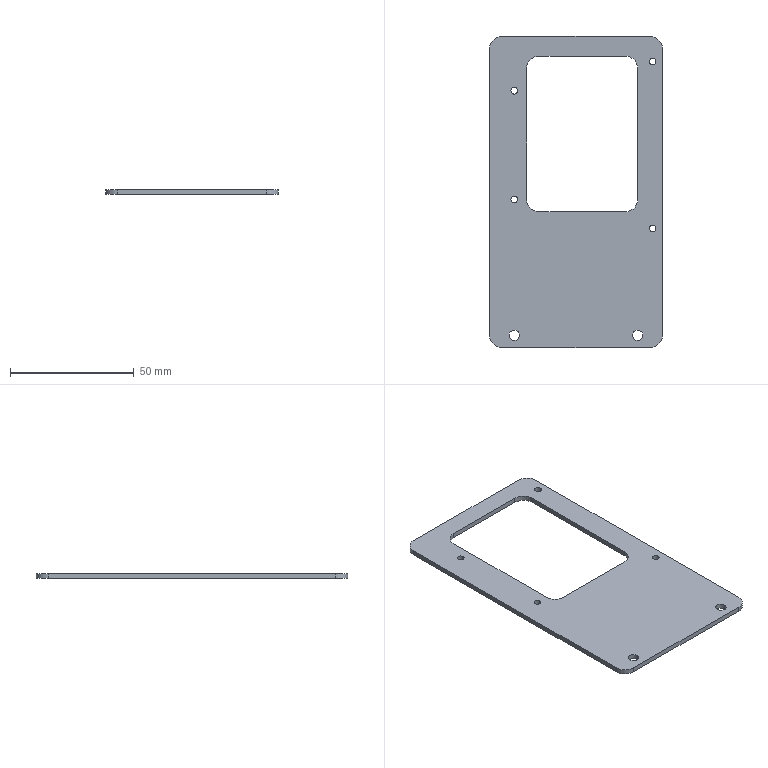Part | SolidWorks | features BaseBody 1 | 1 solid | 30 faces | box 70 x 126 x 2 mm | volume 11869 mm3 | cylinder 20 | plane 10 | commonest cylinder face diameters 2.7 x8 10 x8 4.2 x4
STEP:
#1=CARTESIAN_POINT('',(-27.1,-58.,0.));
#2=VERTEX_POINT('',#1);
#3=CARTESIAN_POINT('',(-22.9,-58.,0.));
#4=VERTEX_POINT('',#3);
#5=CARTESIAN_POINT('',(-25.,-58.,0.));
#6=DIRECTION('',(0.,0.,1.));
#7=DIRECTION('',(1.,0.,0.));
#8=AXIS2_PLACEMENT_3D('',#5,#6,#7);
#9=CIRCLE('',#8,2.1);
#10=EDGE_CURVE('',#2,#4,#9,.T.);
#11=ORIENTED_EDGE('',*,*,#10,.F.);
#12=CARTESIAN_POINT('',(-27.1,-58.,2.));
#13=VERTEX_POINT('',#12);
#14=CARTESIAN_POINT('',(-27.1,-58.,0.));
#15=DIRECTION('',(0.,0.,1.));
#16=VECTOR('',#15,1000.);
#17=LINE('',#14,#16);
#18=EDGE_CURVE('',#2,#13,#17,.T.);
#19=ORIENTED_EDGE('',*,*,#18,.T.);
#20=CARTESIAN_POINT('',(-22.9,-58.,2.));
#21=VERTEX_POINT('',#20);
#22=CARTESIAN_POINT('',(-25.,-58.,2.));
#23=DIRECTION('',(0.,0.,1.));
#24=DIRECTION('',(1.,0.,0.));
#25=AXIS2_PLACEMENT_3D('',#22,#23,#24);
#26=CIRCLE('',#25,2.1);
#27=EDGE_CURVE('',#13,#21,#26,.T.);
#28=ORIENTED_EDGE('',*,*,#27,.T.);
#29=CARTESIAN_POINT('',(-22.9,-58.,0.));
#30=DIRECTION('',(0.,0.,1.));
#31=VECTOR('',#30,1000.);
#32=LINE('',#29,#31);
#33=EDGE_CURVE('',#4,#21,#32,.T.);
#34=ORIENTED_EDGE('',*,*,#33,.F.);
#35=EDGE_LOOP('',(#11,#19,#28,#34));
#36=FACE_OUTER_BOUND('',#35,.T.);
#37=CARTESIAN_POINT('',(-25.,-58.,0.));
#38=DIRECTION('',(0.,0.,1.));
#39=DIRECTION('',(1.,0.,0.));
#40=AXIS2_PLACEMENT_3D('',#37,#38,#39);
#41=CYLINDRICAL_SURFACE('',#40,2.1);
#42=ADVANCED_FACE('',(#36),#41,.F.);
#43=CARTESIAN_POINT('',(29.65,-14.75,0.));
#44=VERTEX_POINT('',#43);
#45=CARTESIAN_POINT('',(32.35,-14.75,0.));
#46=VERTEX_POINT('',#45);
#47=CARTESIAN_POINT('',(31.,-14.75,0.));
#48=DIRECTION('',(0.,0.,1.));
#49=DIRECTION('',(1.,0.,0.));
#50=AXIS2_PLACEMENT_3D('',#47,#48,#49);
#51=CIRCLE('',#50,1.35);
#52=EDGE_CURVE('',#44,#46,#51,.T.);
#53=ORIENTED_EDGE('',*,*,#52,.F.);
#54=CARTESIAN_POINT('',(29.65,-14.75,2.));
#55=VERTEX_POINT('',#54);
#56=CARTESIAN_POINT('',(29.65,-14.75,0.));
#57=DIRECTION('',(0.,0.,1.));
#58=VECTOR('',#57,1000.);
#59=LINE('',#56,#58);
#60=EDGE_CURVE('',#44,#55,#59,.T.);
#61=ORIENTED_EDGE('',*,*,#60,.T.);
#62=CARTESIAN_POINT('',(32.35,-14.75,2.));
#63=VERTEX_POINT('',#62);
#64=CARTESIAN_POINT('',(31.,-14.75,2.));
#65=DIRECTION('',(0.,0.,1.));
#66=DIRECTION('',(1.,0.,0.));
#67=AXIS2_PLACEMENT_3D('',#64,#65,#66);
#68=CIRCLE('',#67,1.35);
#69=EDGE_CURVE('',#55,#63,#68,.T.);
#70=ORIENTED_EDGE('',*,*,#69,.T.);
#71=CARTESIAN_POINT('',(32.35,-14.75,0.));
#72=DIRECTION('',(0.,0.,1.));
#73=VECTOR('',#72,1000.);
#74=LINE('',#71,#73);
#75=EDGE_CURVE('',#46,#63,#74,.T.);
#76=ORIENTED_EDGE('',*,*,#75,.F.);
#77=EDGE_LOOP('',(#53,#61,#70,#76));
#78=FACE_OUTER_BOUND('',#77,.T.);
#79=CARTESIAN_POINT('',(31.,-14.75,0.));
#80=DIRECTION('',(0.,0.,1.));
#81=DIRECTION('',(1.,0.,0.));
#82=AXIS2_PLACEMENT_3D('',#79,#80,#81);
#83=CYLINDRICAL_SURFACE('',#82,1.35);
#84=ADVANCED_FACE('',(#78),#83,.F.);
#85=CARTESIAN_POINT('',(-26.35,41.,0.));
#86=VERTEX_POINT('',#85);
#87=CARTESIAN_POINT('',(-23.65,41.,0.));
#88=VERTEX_POINT('',#87);
#89=CARTESIAN_POINT('',(-25.,41.,0.));
#90=DIRECTION('',(0.,0.,1.));
#91=DIRECTION('',(1.,0.,0.));
#92=AXIS2_PLACEMENT_3D('',#89,#90,#91);
#93=CIRCLE('',#92,1.35);
#94=EDGE_CURVE('',#86,#88,#93,.T.);
#95=ORIENTED_EDGE('',*,*,#94,.F.);
#96=CARTESIAN_POINT('',(-26.35,41.,2.));
#97=VERTEX_POINT('',#96);
#98=CARTESIAN_POINT('',(-26.35,41.,0.));
#99=DIRECTION('',(0.,0.,1.));
#100=VECTOR('',#99,1000.);
#101=LINE('',#98,#100);
#102=EDGE_CURVE('',#86,#97,#101,.T.);
#103=ORIENTED_EDGE('',*,*,#102,.T.);
#104=CARTESIAN_POINT('',(-23.65,41.,2.));
#105=VERTEX_POINT('',#104);
#106=CARTESIAN_POINT('',(-25.,41.,2.));
#107=DIRECTION('',(0.,0.,1.));
#108=DIRECTION('',(1.,0.,0.));
#109=AXIS2_PLACEMENT_3D('',#106,#107,#108);
#110=CIRCLE('',#109,1.35);
#111=EDGE_CURVE('',#97,#105,#110,.T.);
#112=ORIENTED_EDGE('',*,*,#111,.T.);
#113=CARTESIAN_POINT('',(-23.65,41.,0.));
#114=DIRECTION('',(0.,0.,1.));
#115=VECTOR('',#114,1000.);
#116=LINE('',#113,#115);
#117=EDGE_CURVE('',#88,#105,#116,.T.);
#118=ORIENTED_EDGE('',*,*,#117,.F.);
#119=EDGE_LOOP('',(#95,#103,#112,#118));
#120=FACE_OUTER_BOUND('',#119,.T.);
#121=CARTESIAN_POINT('',(-25.,41.,0.));
#122=DIRECTION('',(0.,0.,1.));
#123=DIRECTION('',(1.,0.,0.));
#124=AXIS2_PLACEMENT_3D('',#121,#122,#123);
#125=CYLINDRICAL_SURFACE('',#124,1.35);
#126=ADVANCED_FACE('',(#120),#125,.F.);
#127=CARTESIAN_POINT('',(-26.35,-3.,0.));
#128=VERTEX_POINT('',#127);
#129=CARTESIAN_POINT('',(-23.65,-3.,0.));
#130=VERTEX_POINT('',#129);
#131=CARTESIAN_POINT('',(-25.,-3.,0.));
#132=DIRECTION('',(0.,0.,1.));
#133=DIRECTION('',(1.,0.,0.));
#134=AXIS2_PLACEMENT_3D('',#131,#132,#133);
#135=CIRCLE('',#134,1.35);
#136=EDGE_CURVE('',#128,#130,#135,.T.);
#137=ORIENTED_EDGE('',*,*,#136,.F.);
#138=CARTESIAN_POINT('',(-26.35,-3.,2.));
#139=VERTEX_POINT('',#138);
#140=CARTESIAN_POINT('',(-26.35,-3.,0.));
#141=DIRECTION('',(0.,0.,1.));
#142=VECTOR('',#141,1000.);
#143=LINE('',#140,#142);
#144=EDGE_CURVE('',#128,#139,#143,.T.);
#145=ORIENTED_EDGE('',*,*,#144,.T.);
#146=CARTESIAN_POINT('',(-23.65,-3.,2.));
#147=VERTEX_POINT('',#146);
#148=CARTESIAN_POINT('',(-25.,-3.,2.));
#149=DIRECTION('',(0.,0.,1.));
#150=DIRECTION('',(1.,0.,0.));
#151=AXIS2_PLACEMENT_3D('',#148,#149,#150);
#152=CIRCLE('',#151,1.35);
#153=EDGE_CURVE('',#139,#147,#152,.T.);
#154=ORIENTED_EDGE('',*,*,#153,.T.);
#155=CARTESIAN_POINT('',(-23.65,-3.,0.));
#156=DIRECTION('',(0.,0.,1.));
#157=VECTOR('',#156,1000.);
#158=LINE('',#155,#157);
#159=EDGE_CURVE('',#130,#147,#158,.T.);
#160=ORIENTED_EDGE('',*,*,#159,.F.);
#161=EDGE_LOOP('',(#137,#145,#154,#160));
#162=FACE_OUTER_BOUND('',#161,.T.);
#163=CARTESIAN_POINT('',(-25.,-3.,0.));
#164=DIRECTION('',(0.,0.,1.));
#165=DIRECTION('',(1.,0.,0.));
#166=AXIS2_PLACEMENT_3D('',#163,#164,#165);
#167=CYLINDRICAL_SURFACE('',#166,1.35);
#168=ADVANCED_FACE('',(#162),#167,.F.);
#169=CARTESIAN_POINT('',(22.9,-58.,0.));
#170=VERTEX_POINT('',#169);
#171=CARTESIAN_POINT('',(27.1,-58.,0.));
#172=VERTEX_POINT('',#171);
#173=CARTESIAN_POINT('',(25.,-58.,0.));
#174=DIRECTION('',(0.,0.,1.));
#175=DIRECTION('',(1.,0.,0.));
#176=AXIS2_PLACEMENT_3D('',#173,#174,#175);
#177=CIRCLE('',#176,2.1);
#178=EDGE_CURVE('',#170,#172,#177,.T.);
#179=ORIENTED_EDGE('',*,*,#178,.F.);
#180=CARTESIAN_POINT('',(22.9,-58.,2.));
#181=VERTEX_POINT('',#180);
#182=CARTESIAN_POINT('',(22.9,-58.,0.));
#183=DIRECTION('',(0.,0.,1.));
#184=VECTOR('',#183,1000.);
#185=LINE('',#182,#184);
#186=EDGE_CURVE('',#170,#181,#185,.T.);
#187=ORIENTED_EDGE('',*,*,#186,.T.);
#188=CARTESIAN_POINT('',(27.1,-58.,2.));
#189=VERTEX_POINT('',#188);
#190=CARTESIAN_POINT('',(25.,-58.,2.));
#191=DIRECTION('',(0.,0.,1.));
#192=DIRECTION('',(1.,0.,0.));
#193=AXIS2_PLACEMENT_3D('',#190,#191,#192);
#194=CIRCLE('',#193,2.1);
#195=EDGE_CURVE('',#181,#189,#194,.T.);
#196=ORIENTED_EDGE('',*,*,#195,.T.);
#197=CARTESIAN_POINT('',(27.1,-58.,0.));
#198=DIRECTION('',(0.,0.,1.));
#199=VECTOR('',#198,1000.);
#200=LINE('',#197,#199);
#201=EDGE_CURVE('',#172,#189,#200,.T.);
#202=ORIENTED_EDGE('',*,*,#201,.F.);
#203=EDGE_LOOP('',(#179,#187,#196,#202));
#204=FACE_OUTER_BOUND('',#203,.T.);
#205=CARTESIAN_POINT('',(25.,-58.,0.));
#206=DIRECTION('',(0.,0.,1.));
#207=DIRECTION('',(1.,0.,0.));
#208=AXIS2_PLACEMENT_3D('',#205,#206,#207);
#209=CYLINDRICAL_SURFACE('',#208,2.1);
#210=ADVANCED_FACE('',(#204),#209,.F.);
#211=CARTESIAN_POINT('',(29.65,52.75,0.));
#212=VERTEX_POINT('',#211);
#213=CARTESIAN_POINT('',(32.35,52.75,0.));
#214=VERTEX_POINT('',#213);
#215=CARTESIAN_POINT('',(31.,52.75,0.));
#216=DIRECTION('',(0.,0.,1.));
#217=DIRECTION('',(1.,0.,0.));
#218=AXIS2_PLACEMENT_3D('',#215,#216,#217);
#219=CIRCLE('',#218,1.35);
#220=EDGE_CURVE('',#212,#214,#219,.T.);
#221=ORIENTED_EDGE('',*,*,#220,.F.);
#222=CARTESIAN_POINT('',(29.65,52.75,2.));
#223=VERTEX_POINT('',#222);
#224=CARTESIAN_POINT('',(29.65,52.75,0.));
#225=DIRECTION('',(0.,0.,1.));
#226=VECTOR('',#225,1000.);
#227=LINE('',#224,#226);
#228=EDGE_CURVE('',#212,#223,#227,.T.);
#229=ORIENTED_EDGE('',*,*,#228,.T.);
#230=CARTESIAN_POINT('',(32.35,52.75,2.));
#231=VERTEX_POINT('',#230);
#232=CARTESIAN_POINT('',(31.,52.75,2.));
#233=DIRECTION('',(0.,0.,1.));
#234=DIRECTION('',(1.,0.,0.));
#235=AXIS2_PLACEMENT_3D('',#232,#233,#234);
#236=CIRCLE('',#235,1.35);
#237=EDGE_CURVE('',#223,#231,#236,.T.);
#238=ORIENTED_EDGE('',*,*,#237,.T.);
#239=CARTESIAN_POINT('',(32.35,52.75,0.));
#240=DIRECTION('',(0.,0.,1.));
#241=VECTOR('',#240,1000.);
#242=LINE('',#239,#241);
#243=EDGE_CURVE('',#214,#231,#242,.T.);
#244=ORIENTED_EDGE('',*,*,#243,.F.);
#245=EDGE_LOOP('',(#221,#229,#238,#244));
#246=FACE_OUTER_BOUND('',#245,.T.);
#247=CARTESIAN_POINT('',(31.,52.75,0.));
#248=DIRECTION('',(0.,0.,1.));
#249=DIRECTION('',(1.,0.,0.));
#250=AXIS2_PLACEMENT_3D('',#247,#248,#249);
#251=CYLINDRICAL_SURFACE('',#250,1.35);
#252=ADVANCED_FACE('',(#246),#251,.F.);
#253=CARTESIAN_POINT('',(35.,-58.,2.));
#254=VERTEX_POINT('',#253);
#255=CARTESIAN_POINT('',(30.,-63.,2.));
#256=VERTEX_POINT('',#255);
#257=CARTESIAN_POINT('',(30.,-58.,2.));
#258=DIRECTION('',(0.,0.,-1.));
#259=DIRECTION('',(-1.,0.,0.));
#260=AXIS2_PLACEMENT_3D('',#257,#258,#259);
#261=CIRCLE('',#260,5.);
#262=EDGE_CURVE('',#254,#256,#261,.T.);
#263=ORIENTED_EDGE('',*,*,#262,.F.);
#264=CARTESIAN_POINT('',(35.,58.,2.));
#265=VERTEX_POINT('',#264);
#266=CARTESIAN_POINT('',(35.,0.,2.));
#267=DIRECTION('',(0.,-1.,0.));
#268=VECTOR('',#267,1000.);
#269=LINE('',#266,#268);
#270=EDGE_CURVE('',#265,#254,#269,.T.);
#271=ORIENTED_EDGE('',*,*,#270,.F.);
#272=CARTESIAN_POINT('',(30.,63.,2.));
#273=VERTEX_POINT('',#272);
#274=CARTESIAN_POINT('',(30.,58.,2.));
#275=DIRECTION('',(0.,0.,-1.));
#276=DIRECTION('',(-1.,0.,0.));
#277=AXIS2_PLACEMENT_3D('',#274,#275,#276);
#278=CIRCLE('',#277,5.);
#279=EDGE_CURVE('',#273,#265,#278,.T.);
#280=ORIENTED_EDGE('',*,*,#279,.F.);
#281=CARTESIAN_POINT('',(-30.,63.,2.));
#282=VERTEX_POINT('',#281);
#283=CARTESIAN_POINT('',(0.,63.,2.));
#284=DIRECTION('',(1.,0.,0.));
#285=VECTOR('',#284,1000.);
#286=LINE('',#283,#285);
#287=EDGE_CURVE('',#282,#273,#286,.T.);
#288=ORIENTED_EDGE('',*,*,#287,.F.);
#289=CARTESIAN_POINT('',(-35.,58.,2.));
#290=VERTEX_POINT('',#289);
#291=CARTESIAN_POINT('',(-30.,58.,2.));
#292=DIRECTION('',(0.,0.,-1.));
#293=DIRECTION('',(-1.,0.,0.));
#294=AXIS2_PLACEMENT_3D('',#291,#292,#293);
#295=CIRCLE('',#294,5.);
#296=EDGE_CURVE('',#290,#282,#295,.T.);
#297=ORIENTED_EDGE('',*,*,#296,.F.);
#298=CARTESIAN_POINT('',(-35.,-58.,2.));
#299=VERTEX_POINT('',#298);
#300=CARTESIAN_POINT('',(-35.,0.,2.));
#301=DIRECTION('',(0.,1.,0.));
#302=VECTOR('',#301,1000.);
#303=LINE('',#300,#302);
#304=EDGE_CURVE('',#299,#290,#303,.T.);
#305=ORIENTED_EDGE('',*,*,#304,.F.);
#306=CARTESIAN_POINT('',(-30.,-63.,2.));
#307=VERTEX_POINT('',#306);
#308=CARTESIAN_POINT('',(-30.,-58.,2.));
#309=DIRECTION('',(0.,0.,-1.));
#310=DIRECTION('',(-1.,0.,0.));
#311=AXIS2_PLACEMENT_3D('',#308,#309,#310);
#312=CIRCLE('',#311,5.);
#313=EDGE_CURVE('',#307,#299,#312,.T.);
#314=ORIENTED_EDGE('',*,*,#313,.F.);
#315=CARTESIAN_POINT('',(0.,-63.,2.));
#316=DIRECTION('',(-1.,0.,0.));
#317=VECTOR('',#316,1000.);
#318=LINE('',#315,#317);
#319=EDGE_CURVE('',#256,#307,#318,.T.);
#320=ORIENTED_EDGE('',*,*,#319,.F.);
#321=EDGE_LOOP('',(#263,#271,#280,#288,#297,#305,#314,#320));
#322=FACE_OUTER_BOUND('',#321,.T.);
#323=CARTESIAN_POINT('',(-25.,-58.,2.));
#324=DIRECTION('',(0.,0.,1.));
#325=DIRECTION('',(1.,0.,0.));
#326=AXIS2_PLACEMENT_3D('',#323,#324,#325);
#327=CIRCLE('',#326,2.1);
#328=EDGE_CURVE('',#21,#13,#327,.T.);
#329=ORIENTED_EDGE('',*,*,#328,.F.);
#330=ORIENTED_EDGE('',*,*,#27,.F.);
#331=EDGE_LOOP('',(#329,#330));
#332=FACE_BOUND('',#331,.T.);
#333=CARTESIAN_POINT('',(31.,-14.75,2.));
#334=DIRECTION('',(0.,0.,1.));
#335=DIRECTION('',(1.,0.,0.));
#336=AXIS2_PLACEMENT_3D('',#333,#334,#335);
#337=CIRCLE('',#336,1.35);
#338=EDGE_CURVE('',#63,#55,#337,.T.);
#339=ORIENTED_EDGE('',*,*,#338,.F.);
#340=ORIENTED_EDGE('',*,*,#69,.F.);
#341=EDGE_LOOP('',(#339,#340));
#342=FACE_BOUND('',#341,.T.);
#343=CARTESIAN_POINT('',(-25.,41.,2.));
#344=DIRECTION('',(0.,0.,1.));
#345=DIRECTION('',(1.,0.,0.));
#346=AXIS2_PLACEMENT_3D('',#343,#344,#345);
#347=CIRCLE('',#346,1.35);
#348=EDGE_CURVE('',#105,#97,#347,.T.);
#349=ORIENTED_EDGE('',*,*,#348,.F.);
#350=ORIENTED_EDGE('',*,*,#111,.F.);
#351=EDGE_LOOP('',(#349,#350));
#352=FACE_BOUND('',#351,.T.);
#353=CARTESIAN_POINT('',(-25.,-3.,2.));
#354=DIRECTION('',(0.,0.,1.));
#355=DIRECTION('',(1.,0.,0.));
#356=AXIS2_PLACEMENT_3D('',#353,#354,#355);
#357=CIRCLE('',#356,1.35);
#358=EDGE_CURVE('',#147,#139,#357,.T.);
#359=ORIENTED_EDGE('',*,*,#358,.F.);
#360=ORIENTED_EDGE('',*,*,#153,.F.);
#361=EDGE_LOOP('',(#359,#360));
#362=FACE_BOUND('',#361,.T.);
#363=CARTESIAN_POINT('',(25.,-58.,2.));
#364=DIRECTION('',(0.,0.,1.));
#365=DIRECTION('',(1.,0.,0.));
#366=AXIS2_PLACEMENT_3D('',#363,#364,#365);
#367=CIRCLE('',#366,2.1);
#368=EDGE_CURVE('',#189,#181,#367,.T.);
#369=ORIENTED_EDGE('',*,*,#368,.F.);
#370=ORIENTED_EDGE('',*,*,#195,.F.);
#371=EDGE_LOOP('',(#369,#370));
#372=FACE_BOUND('',#371,.T.);
#373=CARTESIAN_POINT('',(31.,52.75,2.));
#374=DIRECTION('',(0.,0.,1.));
#375=DIRECTION('',(1.,0.,0.));
#376=AXIS2_PLACEMENT_3D('',#373,#374,#375);
#377=CIRCLE('',#376,1.35);
#378=EDGE_CURVE('',#231,#223,#377,.T.);
#379=ORIENTED_EDGE('',*,*,#378,.F.);
#380=ORIENTED_EDGE('',*,*,#237,.F.);
#381=EDGE_LOOP('',(#379,#380));
#382=FACE_BOUND('',#381,.T.);
#383=CARTESIAN_POINT('',(25.,50.,2.));
#384=VERTEX_POINT('',#383);
#385=CARTESIAN_POINT('',(20.,55.,2.));
#386=VERTEX_POINT('',#385);
#387=CARTESIAN_POINT('',(20.,50.,2.));
#388=DIRECTION('',(0.,0.,1.));
#389=DIRECTION('',(-1.,0.,0.));
#390=AXIS2_PLACEMENT_3D('',#387,#388,#389);
#391=CIRCLE('',#390,5.);
#392=EDGE_CURVE('',#384,#386,#391,.T.);
#393=ORIENTED_EDGE('',*,*,#392,.F.);
#394=CARTESIAN_POINT('',(25.,-3.,2.));
#395=VERTEX_POINT('',#394);
#396=CARTESIAN_POINT('',(25.,0.,2.));
#397=DIRECTION('',(0.,1.,0.));
#398=VECTOR('',#397,1000.);
#399=LINE('',#396,#398);
#400=EDGE_CURVE('',#395,#384,#399,.T.);
#401=ORIENTED_EDGE('',*,*,#400,.F.);
#402=CARTESIAN_POINT('',(20.,-8.,2.));
#403=VERTEX_POINT('',#402);
#404=CARTESIAN_POINT('',(20.,-3.,2.));
#405=DIRECTION('',(0.,0.,1.));
#406=DIRECTION('',(-1.,0.,0.));
#407=AXIS2_PLACEMENT_3D('',#404,#405,#406);
#408=CIRCLE('',#407,5.);
#409=EDGE_CURVE('',#403,#395,#408,.T.);
#410=ORIENTED_EDGE('',*,*,#409,.F.);
#411=CARTESIAN_POINT('',(-15.,-8.,2.));
#412=VERTEX_POINT('',#411);
#413=CARTESIAN_POINT('',(0.,-8.,2.));
#414=DIRECTION('',(1.,0.,0.));
#415=VECTOR('',#414,1000.);
#416=LINE('',#413,#415);
#417=EDGE_CURVE('',#412,#403,#416,.T.);
#418=ORIENTED_EDGE('',*,*,#417,.F.);
#419=CARTESIAN_POINT('',(-20.,-3.,2.));
#420=VERTEX_POINT('',#419);
#421=CARTESIAN_POINT('',(-15.,-3.,2.));
#422=DIRECTION('',(0.,0.,1.));
#423=DIRECTION('',(-1.,0.,0.));
#424=AXIS2_PLACEMENT_3D('',#421,#422,#423);
#425=CIRCLE('',#424,5.);
#426=EDGE_CURVE('',#420,#412,#425,.T.);
#427=ORIENTED_EDGE('',*,*,#426,.F.);
#428=CARTESIAN_POINT('',(-20.,50.,2.));
#429=VERTEX_POINT('',#428);
#430=CARTESIAN_POINT('',(-20.,0.,2.));
#431=DIRECTION('',(0.,-1.,0.));
#432=VECTOR('',#431,1000.);
#433=LINE('',#430,#432);
#434=EDGE_CURVE('',#429,#420,#433,.T.);
#435=ORIENTED_EDGE('',*,*,#434,.F.);
#436=CARTESIAN_POINT('',(-15.,55.,2.));
#437=VERTEX_POINT('',#436);
#438=CARTESIAN_POINT('',(-15.,50.,2.));
#439=DIRECTION('',(0.,0.,1.));
#440=DIRECTION('',(-1.,0.,0.));
#441=AXIS2_PLACEMENT_3D('',#438,#439,#440);
#442=CIRCLE('',#441,5.);
#443=EDGE_CURVE('',#437,#429,#442,.T.);
#444=ORIENTED_EDGE('',*,*,#443,.F.);
#445=CARTESIAN_POINT('',(0.,55.,2.));
#446=DIRECTION('',(-1.,0.,0.));
#447=VECTOR('',#446,1000.);
#448=LINE('',#445,#447);
#449=EDGE_CURVE('',#386,#437,#448,.T.);
#450=ORIENTED_EDGE('',*,*,#449,.F.);
#451=EDGE_LOOP('',(#393,#401,#410,#418,#427,#435,#444,#450));
#452=FACE_BOUND('',#451,.T.);
#453=CARTESIAN_POINT('',(0.,0.,2.));
#454=DIRECTION('',(0.,0.,-1.));
#455=DIRECTION('',(-1.,0.,0.));
#456=AXIS2_PLACEMENT_3D('',#453,#454,#455);
#457=PLANE('',#456);
#458=ADVANCED_FACE('',(#322,#332,#342,#352,#362,#372,#382,#452),#457,.F.);
#459=CARTESIAN_POINT('',(30.,-63.,0.));
#460=VERTEX_POINT('',#459);
#461=CARTESIAN_POINT('',(30.,-63.,2.));
#462=DIRECTION('',(0.,0.,-1.));
#463=VECTOR('',#462,1000.);
#464=LINE('',#461,#463);
#465=EDGE_CURVE('',#256,#460,#464,.T.);
#466=ORIENTED_EDGE('',*,*,#465,.F.);
#467=ORIENTED_EDGE('',*,*,#319,.T.);
#468=CARTESIAN_POINT('',(-30.,-63.,0.));
#469=VERTEX_POINT('',#468);
#470=CARTESIAN_POINT('',(-30.,-63.,2.));
#471=DIRECTION('',(0.,0.,1.));
#472=VECTOR('',#471,1000.);
#473=LINE('',#470,#472);
#474=EDGE_CURVE('',#469,#307,#473,.T.);
#475=ORIENTED_EDGE('',*,*,#474,.F.);
#476=CARTESIAN_POINT('',(-35.,-63.,0.));
#477=DIRECTION('',(-1.,0.,0.));
#478=VECTOR('',#477,1000.);
#479=LINE('',#476,#478);
#480=EDGE_CURVE('',#460,#469,#479,.T.);
#481=ORIENTED_EDGE('',*,*,#480,.F.);
#482=EDGE_LOOP('',(#466,#467,#475,#481));
#483=FACE_OUTER_BOUND('',#482,.T.);
#484=CARTESIAN_POINT('',(-35.,-63.,2.));
#485=DIRECTION('',(0.,1.,0.));
#486=DIRECTION('',(0.,0.,1.));
#487=AXIS2_PLACEMENT_3D('',#484,#485,#486);
#488=PLANE('',#487);
#489=ADVANCED_FACE('',(#483),#488,.F.);
#490=CARTESIAN_POINT('',(35.,-58.,0.));
#491=VERTEX_POINT('',#490);
#492=CARTESIAN_POINT('',(30.,-58.,0.));
#493=DIRECTION('',(0.,0.,1.));
#494=DIRECTION('',(-1.,0.,0.));
#495=AXIS2_PLACEMENT_3D('',#492,#493,#494);
#496=CIRCLE('',#495,5.);
#497=EDGE_CURVE('',#460,#491,#496,.T.);
#498=ORIENTED_EDGE('',*,*,#497,.T.);
#499=CARTESIAN_POINT('',(35.,-58.,2.));
#500=DIRECTION('',(0.,0.,1.));
#501=VECTOR('',#500,1000.);
#502=LINE('',#499,#501);
#503=EDGE_CURVE('',#491,#254,#502,.T.);
#504=ORIENTED_EDGE('',*,*,#503,.T.);
#505=ORIENTED_EDGE('',*,*,#262,.T.);
#506=ORIENTED_EDGE('',*,*,#465,.T.);
#507=EDGE_LOOP('',(#498,#504,#505,#506));
#508=FACE_OUTER_BOUND('',#507,.T.);
#509=CARTESIAN_POINT('',(30.,-58.,2.));
#510=DIRECTION('',(0.,0.,-1.));
#511=DIRECTION('',(-1.,0.,0.));
#512=AXIS2_PLACEMENT_3D('',#509,#510,#511);
#513=CYLINDRICAL_SURFACE('',#512,5.);
#514=ADVANCED_FACE('',(#508),#513,.T.);
#515=ORIENTED_EDGE('',*,*,#503,.F.);
#516=CARTESIAN_POINT('',(35.,58.,0.));
#517=VERTEX_POINT('',#516);
#518=CARTESIAN_POINT('',(35.,-63.,0.));
#519=DIRECTION('',(0.,-1.,0.));
#520=VECTOR('',#519,1000.);
#521=LINE('',#518,#520);
#522=EDGE_CURVE('',#517,#491,#521,.T.);
#523=ORIENTED_EDGE('',*,*,#522,.F.);
#524=CARTESIAN_POINT('',(35.,58.,2.));
#525=DIRECTION('',(0.,0.,-1.));
#526=VECTOR('',#525,1000.);
#527=LINE('',#524,#526);
#528=EDGE_CURVE('',#265,#517,#527,.T.);
#529=ORIENTED_EDGE('',*,*,#528,.F.);
#530=ORIENTED_EDGE('',*,*,#270,.T.);
#531=EDGE_LOOP('',(#515,#523,#529,#530));
#532=FACE_OUTER_BOUND('',#531,.T.);
#533=CARTESIAN_POINT('',(35.,-63.,2.));
#534=DIRECTION('',(-1.,0.,0.));
#535=DIRECTION('',(0.,0.,1.));
#536=AXIS2_PLACEMENT_3D('',#533,#534,#535);
#537=PLANE('',#536);
#538=ADVANCED_FACE('',(#532),#537,.F.);
#539=CARTESIAN_POINT('',(30.,63.,0.));
#540=VERTEX_POINT('',#539);
#541=CARTESIAN_POINT('',(30.,58.,0.));
#542=DIRECTION('',(0.,0.,1.));
#543=DIRECTION('',(-1.,0.,0.));
#544=AXIS2_PLACEMENT_3D('',#541,#542,#543);
#545=CIRCLE('',#544,5.);
#546=EDGE_CURVE('',#517,#540,#545,.T.);
#547=ORIENTED_EDGE('',*,*,#546,.T.);
#548=CARTESIAN_POINT('',(30.,63.,2.));
#549=DIRECTION('',(0.,0.,1.));
#550=VECTOR('',#549,1000.);
#551=LINE('',#548,#550);
#552=EDGE_CURVE('',#540,#273,#551,.T.);
#553=ORIENTED_EDGE('',*,*,#552,.T.);
#554=ORIENTED_EDGE('',*,*,#279,.T.);
#555=ORIENTED_EDGE('',*,*,#528,.T.);
#556=EDGE_LOOP('',(#547,#553,#554,#555));
#557=FACE_OUTER_BOUND('',#556,.T.);
#558=CARTESIAN_POINT('',(30.,58.,2.));
#559=DIRECTION('',(0.,0.,-1.));
#560=DIRECTION('',(-1.,0.,0.));
#561=AXIS2_PLACEMENT_3D('',#558,#559,#560);
#562=CYLINDRICAL_SURFACE('',#561,5.);
#563=ADVANCED_FACE('',(#557),#562,.T.);
#564=ORIENTED_EDGE('',*,*,#552,.F.);
#565=CARTESIAN_POINT('',(-30.,63.,0.));
#566=VERTEX_POINT('',#565);
#567=CARTESIAN_POINT('',(-35.,63.,0.));
#568=DIRECTION('',(1.,0.,0.));
#569=VECTOR('',#568,1000.);
#570=LINE('',#567,#569);
#571=EDGE_CURVE('',#566,#540,#570,.T.);
#572=ORIENTED_EDGE('',*,*,#571,.F.);
#573=CARTESIAN_POINT('',(-30.,63.,2.));
#574=DIRECTION('',(0.,0.,-1.));
#575=VECTOR('',#574,1000.);
#576=LINE('',#573,#575);
#577=EDGE_CURVE('',#282,#566,#576,.T.);
#578=ORIENTED_EDGE('',*,*,#577,.F.);
#579=ORIENTED_EDGE('',*,*,#287,.T.);
#580=EDGE_LOOP('',(#564,#572,#578,#579));
#581=FACE_OUTER_BOUND('',#580,.T.);
#582=CARTESIAN_POINT('',(-35.,63.,2.));
#583=DIRECTION('',(0.,-1.,0.));
#584=DIRECTION('',(0.,0.,-1.));
#585=AXIS2_PLACEMENT_3D('',#582,#583,#584);
#586=PLANE('',#585);
#587=ADVANCED_FACE('',(#581),#586,.F.);
#588=CARTESIAN_POINT('',(-35.,58.,0.));
#589=VERTEX_POINT('',#588);
#590=CARTESIAN_POINT('',(-30.,58.,0.));
#591=DIRECTION('',(0.,0.,1.));
#592=DIRECTION('',(-1.,0.,0.));
#593=AXIS2_PLACEMENT_3D('',#590,#591,#592);
#594=CIRCLE('',#593,5.);
#595=EDGE_CURVE('',#566,#589,#594,.T.);
#596=ORIENTED_EDGE('',*,*,#595,.T.);
#597=CARTESIAN_POINT('',(-35.,58.,2.));
#598=DIRECTION('',(0.,0.,1.));
#599=VECTOR('',#598,1000.);
#600=LINE('',#597,#599);
#601=EDGE_CURVE('',#589,#290,#600,.T.);
#602=ORIENTED_EDGE('',*,*,#601,.T.);
#603=ORIENTED_EDGE('',*,*,#296,.T.);
#604=ORIENTED_EDGE('',*,*,#577,.T.);
#605=EDGE_LOOP('',(#596,#602,#603,#604));
#606=FACE_OUTER_BOUND('',#605,.T.);
#607=CARTESIAN_POINT('',(-30.,58.,2.));
#608=DIRECTION('',(0.,0.,-1.));
#609=DIRECTION('',(-1.,0.,0.));
#610=AXIS2_PLACEMENT_3D('',#607,#608,#609);
#611=CYLINDRICAL_SURFACE('',#610,5.);
#612=ADVANCED_FACE('',(#606),#611,.T.);
#613=CARTESIAN_POINT('',(-35.,-58.,0.));
#614=VERTEX_POINT('',#613);
#615=CARTESIAN_POINT('',(-35.,-58.,2.));
#616=DIRECTION('',(0.,0.,-1.));
#617=VECTOR('',#616,1000.);
#618=LINE('',#615,#617);
#619=EDGE_CURVE('',#299,#614,#618,.T.);
#620=ORIENTED_EDGE('',*,*,#619,.F.);
#621=ORIENTED_EDGE('',*,*,#304,.T.);
#622=ORIENTED_EDGE('',*,*,#601,.F.);
#623=CARTESIAN_POINT('',(-35.,-63.,0.));
#624=DIRECTION('',(0.,1.,0.));
#625=VECTOR('',#624,1000.);
#626=LINE('',#623,#625);
#627=EDGE_CURVE('',#614,#589,#626,.T.);
#628=ORIENTED_EDGE('',*,*,#627,.F.);
#629=EDGE_LOOP('',(#620,#621,#622,#628));
#630=FACE_OUTER_BOUND('',#629,.T.);
#631=CARTESIAN_POINT('',(-35.,-63.,2.));
#632=DIRECTION('',(1.,0.,0.));
#633=DIRECTION('',(0.,0.,-1.));
#634=AXIS2_PLACEMENT_3D('',#631,#632,#633);
#635=PLANE('',#634);
#636=ADVANCED_FACE('',(#630),#635,.F.);
#637=CARTESIAN_POINT('',(-30.,-58.,0.));
#638=DIRECTION('',(0.,0.,1.));
#639=DIRECTION('',(-1.,0.,0.));
#640=AXIS2_PLACEMENT_3D('',#637,#638,#639);
#641=CIRCLE('',#640,5.);
#642=EDGE_CURVE('',#614,#469,#641,.T.);
#643=ORIENTED_EDGE('',*,*,#642,.T.);
#644=ORIENTED_EDGE('',*,*,#474,.T.);
#645=ORIENTED_EDGE('',*,*,#313,.T.);
#646=ORIENTED_EDGE('',*,*,#619,.T.);
#647=EDGE_LOOP('',(#643,#644,#645,#646));
#648=FACE_OUTER_BOUND('',#647,.T.);
#649=CARTESIAN_POINT('',(-30.,-58.,2.));
#650=DIRECTION('',(0.,0.,-1.));
#651=DIRECTION('',(-1.,0.,0.));
#652=AXIS2_PLACEMENT_3D('',#649,#650,#651);
#653=CYLINDRICAL_SURFACE('',#652,5.);
#654=ADVANCED_FACE('',(#648),#653,.T.);
#655=ORIENTED_EDGE('',*,*,#18,.F.);
#656=CARTESIAN_POINT('',(-25.,-58.,0.));
#657=DIRECTION('',(0.,0.,1.));
#658=DIRECTION('',(1.,0.,0.));
#659=AXIS2_PLACEMENT_3D('',#656,#657,#658);
#660=CIRCLE('',#659,2.1);
#661=EDGE_CURVE('',#4,#2,#660,.T.);
#662=ORIENTED_EDGE('',*,*,#661,.F.);
#663=ORIENTED_EDGE('',*,*,#33,.T.);
#664=ORIENTED_EDGE('',*,*,#328,.T.);
#665=EDGE_LOOP('',(#655,#662,#663,#664));
#666=FACE_OUTER_BOUND('',#665,.T.);
#667=CARTESIAN_POINT('',(-25.,-58.,0.));
#668=DIRECTION('',(0.,0.,1.));
#669=DIRECTION('',(1.,0.,0.));
#670=AXIS2_PLACEMENT_3D('',#667,#668,#669);
#671=CYLINDRICAL_SURFACE('',#670,2.1);
#672=ADVANCED_FACE('',(#666),#671,.F.);
#673=ORIENTED_EDGE('',*,*,#60,.F.);
#674=CARTESIAN_POINT('',(31.,-14.75,0.));
#675=DIRECTION('',(0.,0.,1.));
#676=DIRECTION('',(1.,0.,0.));
#677=AXIS2_PLACEMENT_3D('',#674,#675,#676);
#678=CIRCLE('',#677,1.35);
#679=EDGE_CURVE('',#46,#44,#678,.T.);
#680=ORIENTED_EDGE('',*,*,#679,.F.);
#681=ORIENTED_EDGE('',*,*,#75,.T.);
#682=ORIENTED_EDGE('',*,*,#338,.T.);
#683=EDGE_LOOP('',(#673,#680,#681,#682));
#684=FACE_OUTER_BOUND('',#683,.T.);
#685=CARTESIAN_POINT('',(31.,-14.75,0.));
#686=DIRECTION('',(0.,0.,1.));
#687=DIRECTION('',(1.,0.,0.));
#688=AXIS2_PLACEMENT_3D('',#685,#686,#687);
#689=CYLINDRICAL_SURFACE('',#688,1.35);
#690=ADVANCED_FACE('',(#684),#689,.F.);
#691=ORIENTED_EDGE('',*,*,#102,.F.);
#692=CARTESIAN_POINT('',(-25.,41.,0.));
#693=DIRECTION('',(0.,0.,1.));
#694=DIRECTION('',(1.,0.,0.));
#695=AXIS2_PLACEMENT_3D('',#692,#693,#694);
#696=CIRCLE('',#695,1.35);
#697=EDGE_CURVE('',#88,#86,#696,.T.);
#698=ORIENTED_EDGE('',*,*,#697,.F.);
#699=ORIENTED_EDGE('',*,*,#117,.T.);
#700=ORIENTED_EDGE('',*,*,#348,.T.);
#701=EDGE_LOOP('',(#691,#698,#699,#700));
#702=FACE_OUTER_BOUND('',#701,.T.);
#703=CARTESIAN_POINT('',(-25.,41.,0.));
#704=DIRECTION('',(0.,0.,1.));
#705=DIRECTION('',(1.,0.,0.));
#706=AXIS2_PLACEMENT_3D('',#703,#704,#705);
#707=CYLINDRICAL_SURFACE('',#706,1.35);
#708=ADVANCED_FACE('',(#702),#707,.F.);
#709=ORIENTED_EDGE('',*,*,#144,.F.);
#710=CARTESIAN_POINT('',(-25.,-3.,0.));
#711=DIRECTION('',(0.,0.,1.));
#712=DIRECTION('',(1.,0.,0.));
#713=AXIS2_PLACEMENT_3D('',#710,#711,#712);
#714=CIRCLE('',#713,1.35);
#715=EDGE_CURVE('',#130,#128,#714,.T.);
#716=ORIENTED_EDGE('',*,*,#715,.F.);
#717=ORIENTED_EDGE('',*,*,#159,.T.);
#718=ORIENTED_EDGE('',*,*,#358,.T.);
#719=EDGE_LOOP('',(#709,#716,#717,#718));
#720=FACE_OUTER_BOUND('',#719,.T.);
#721=CARTESIAN_POINT('',(-25.,-3.,0.));
#722=DIRECTION('',(0.,0.,1.));
#723=DIRECTION('',(1.,0.,0.));
#724=AXIS2_PLACEMENT_3D('',#721,#722,#723);
#725=CYLINDRICAL_SURFACE('',#724,1.35);
#726=ADVANCED_FACE('',(#720),#725,.F.);
#727=ORIENTED_EDGE('',*,*,#186,.F.);
#728=CARTESIAN_POINT('',(25.,-58.,0.));
#729=DIRECTION('',(0.,0.,1.));
#730=DIRECTION('',(1.,0.,0.));
#731=AXIS2_PLACEMENT_3D('',#728,#729,#730);
#732=CIRCLE('',#731,2.1);
#733=EDGE_CURVE('',#172,#170,#732,.T.);
#734=ORIENTED_EDGE('',*,*,#733,.F.);
#735=ORIENTED_EDGE('',*,*,#201,.T.);
#736=ORIENTED_EDGE('',*,*,#368,.T.);
#737=EDGE_LOOP('',(#727,#734,#735,#736));
#738=FACE_OUTER_BOUND('',#737,.T.);
#739=CARTESIAN_POINT('',(25.,-58.,0.));
#740=DIRECTION('',(0.,0.,1.));
#741=DIRECTION('',(1.,0.,0.));
#742=AXIS2_PLACEMENT_3D('',#739,#740,#741);
#743=CYLINDRICAL_SURFACE('',#742,2.1);
#744=ADVANCED_FACE('',(#738),#743,.F.);
#745=ORIENTED_EDGE('',*,*,#228,.F.);
#746=CARTESIAN_POINT('',(31.,52.75,0.));
#747=DIRECTION('',(0.,0.,1.));
#748=DIRECTION('',(1.,0.,0.));
#749=AXIS2_PLACEMENT_3D('',#746,#747,#748);
#750=CIRCLE('',#749,1.35);
#751=EDGE_CURVE('',#214,#212,#750,.T.);
#752=ORIENTED_EDGE('',*,*,#751,.F.);
#753=ORIENTED_EDGE('',*,*,#243,.T.);
#754=ORIENTED_EDGE('',*,*,#378,.T.);
#755=EDGE_LOOP('',(#745,#752,#753,#754));
#756=FACE_OUTER_BOUND('',#755,.T.);
#757=CARTESIAN_POINT('',(31.,52.75,0.));
#758=DIRECTION('',(0.,0.,1.));
#759=DIRECTION('',(1.,0.,0.));
#760=AXIS2_PLACEMENT_3D('',#757,#758,#759);
#761=CYLINDRICAL_SURFACE('',#760,1.35);
#762=ADVANCED_FACE('',(#756),#761,.F.);
#763=CARTESIAN_POINT('',(-15.,55.,0.));
#764=VERTEX_POINT('',#763);
#765=CARTESIAN_POINT('',(-15.,55.,-8.));
#766=DIRECTION('',(0.,0.,1.));
#767=VECTOR('',#766,1000.);
#768=LINE('',#765,#767);
#769=EDGE_CURVE('',#764,#437,#768,.T.);
#770=ORIENTED_EDGE('',*,*,#769,.F.);
#771=CARTESIAN_POINT('',(20.,55.,0.));
#772=VERTEX_POINT('',#771);
#773=CARTESIAN_POINT('',(-20.,55.,0.));
#774=DIRECTION('',(-1.,0.,0.));
#775=VECTOR('',#774,1000.);
#776=LINE('',#773,#775);
#777=EDGE_CURVE('',#772,#764,#776,.T.);
#778=ORIENTED_EDGE('',*,*,#777,.F.);
#779=CARTESIAN_POINT('',(20.,55.,-8.));
#780=DIRECTION('',(0.,0.,-1.));
#781=VECTOR('',#780,1000.);
#782=LINE('',#779,#781);
#783=EDGE_CURVE('',#386,#772,#782,.T.);
#784=ORIENTED_EDGE('',*,*,#783,.F.);
#785=ORIENTED_EDGE('',*,*,#449,.T.);
#786=EDGE_LOOP('',(#770,#778,#784,#785));
#787=FACE_OUTER_BOUND('',#786,.T.);
#788=CARTESIAN_POINT('',(-20.,55.,-8.));
#789=DIRECTION('',(0.,1.,0.));
#790=DIRECTION('',(0.,0.,1.));
#791=AXIS2_PLACEMENT_3D('',#788,#789,#790);
#792=PLANE('',#791);
#793=ADVANCED_FACE('',(#787),#792,.F.);
#794=CARTESIAN_POINT('',(25.,50.,0.));
#795=VERTEX_POINT('',#794);
#796=CARTESIAN_POINT('',(25.,50.,-8.));
#797=DIRECTION('',(0.,0.,-1.));
#798=VECTOR('',#797,1000.);
#799=LINE('',#796,#798);
#800=EDGE_CURVE('',#384,#795,#799,.T.);
#801=ORIENTED_EDGE('',*,*,#800,.F.);
#802=ORIENTED_EDGE('',*,*,#392,.T.);
#803=ORIENTED_EDGE('',*,*,#783,.T.);
#804=CARTESIAN_POINT('',(20.,50.,0.));
#805=DIRECTION('',(0.,0.,1.));
#806=DIRECTION('',(-1.,0.,0.));
#807=AXIS2_PLACEMENT_3D('',#804,#805,#806);
#808=CIRCLE('',#807,5.);
#809=EDGE_CURVE('',#795,#772,#808,.T.);
#810=ORIENTED_EDGE('',*,*,#809,.F.);
#811=EDGE_LOOP('',(#801,#802,#803,#810));
#812=FACE_OUTER_BOUND('',#811,.T.);
#813=CARTESIAN_POINT('',(20.,50.,-8.));
#814=DIRECTION('',(0.,0.,-1.));
#815=DIRECTION('',(-1.,0.,0.));
#816=AXIS2_PLACEMENT_3D('',#813,#814,#815);
#817=CYLINDRICAL_SURFACE('',#816,5.);
#818=ADVANCED_FACE('',(#812),#817,.F.);
#819=CARTESIAN_POINT('',(25.,-3.,0.));
#820=VERTEX_POINT('',#819);
#821=CARTESIAN_POINT('',(25.,-3.,-8.));
#822=DIRECTION('',(0.,0.,-1.));
#823=VECTOR('',#822,1000.);
#824=LINE('',#821,#823);
#825=EDGE_CURVE('',#395,#820,#824,.T.);
#826=ORIENTED_EDGE('',*,*,#825,.F.);
#827=ORIENTED_EDGE('',*,*,#400,.T.);
#828=ORIENTED_EDGE('',*,*,#800,.T.);
#829=CARTESIAN_POINT('',(25.,-8.,0.));
#830=DIRECTION('',(0.,1.,0.));
#831=VECTOR('',#830,1000.);
#832=LINE('',#829,#831);
#833=EDGE_CURVE('',#820,#795,#832,.T.);
#834=ORIENTED_EDGE('',*,*,#833,.F.);
#835=EDGE_LOOP('',(#826,#827,#828,#834));
#836=FACE_OUTER_BOUND('',#835,.T.);
#837=CARTESIAN_POINT('',(25.,-8.,-8.));
#838=DIRECTION('',(1.,0.,0.));
#839=DIRECTION('',(0.,0.,-1.));
#840=AXIS2_PLACEMENT_3D('',#837,#838,#839);
#841=PLANE('',#840);
#842=ADVANCED_FACE('',(#836),#841,.F.);
#843=CARTESIAN_POINT('',(20.,-8.,0.));
#844=VERTEX_POINT('',#843);
#845=CARTESIAN_POINT('',(20.,-8.,-8.));
#846=DIRECTION('',(0.,0.,-1.));
#847=VECTOR('',#846,1000.);
#848=LINE('',#845,#847);
#849=EDGE_CURVE('',#403,#844,#848,.T.);
#850=ORIENTED_EDGE('',*,*,#849,.F.);
#851=ORIENTED_EDGE('',*,*,#409,.T.);
#852=ORIENTED_EDGE('',*,*,#825,.T.);
#853=CARTESIAN_POINT('',(20.,-3.,0.));
#854=DIRECTION('',(0.,0.,1.));
#855=DIRECTION('',(-1.,0.,0.));
#856=AXIS2_PLACEMENT_3D('',#853,#854,#855);
#857=CIRCLE('',#856,5.);
#858=EDGE_CURVE('',#844,#820,#857,.T.);
#859=ORIENTED_EDGE('',*,*,#858,.F.);
#860=EDGE_LOOP('',(#850,#851,#852,#859));
#861=FACE_OUTER_BOUND('',#860,.T.);
#862=CARTESIAN_POINT('',(20.,-3.,-8.));
#863=DIRECTION('',(0.,0.,-1.));
#864=DIRECTION('',(-1.,0.,0.));
#865=AXIS2_PLACEMENT_3D('',#862,#863,#864);
#866=CYLINDRICAL_SURFACE('',#865,5.);
#867=ADVANCED_FACE('',(#861),#866,.F.);
#868=ORIENTED_EDGE('',*,*,#849,.T.);
#869=CARTESIAN_POINT('',(-15.,-8.,0.));
#870=VERTEX_POINT('',#869);
#871=CARTESIAN_POINT('',(-20.,-8.,0.));
#872=DIRECTION('',(1.,0.,0.));
#873=VECTOR('',#872,1000.);
#874=LINE('',#871,#873);
#875=EDGE_CURVE('',#870,#844,#874,.T.);
#876=ORIENTED_EDGE('',*,*,#875,.F.);
#877=CARTESIAN_POINT('',(-15.,-8.,-8.));
#878=DIRECTION('',(0.,0.,-1.));
#879=VECTOR('',#878,1000.);
#880=LINE('',#877,#879);
#881=EDGE_CURVE('',#412,#870,#880,.T.);
#882=ORIENTED_EDGE('',*,*,#881,.F.);
#883=ORIENTED_EDGE('',*,*,#417,.T.);
#884=EDGE_LOOP('',(#868,#876,#882,#883));
#885=FACE_OUTER_BOUND('',#884,.T.);
#886=CARTESIAN_POINT('',(-20.,-8.,-8.));
#887=DIRECTION('',(0.,-1.,0.));
#888=DIRECTION('',(0.,0.,-1.));
#889=AXIS2_PLACEMENT_3D('',#886,#887,#888);
#890=PLANE('',#889);
#891=ADVANCED_FACE('',(#885),#890,.F.);
#892=CARTESIAN_POINT('',(-20.,-3.,0.));
#893=VERTEX_POINT('',#892);
#894=CARTESIAN_POINT('',(-20.,-3.,-8.));
#895=DIRECTION('',(0.,0.,-1.));
#896=VECTOR('',#895,1000.);
#897=LINE('',#894,#896);
#898=EDGE_CURVE('',#420,#893,#897,.T.);
#899=ORIENTED_EDGE('',*,*,#898,.F.);
#900=ORIENTED_EDGE('',*,*,#426,.T.);
#901=ORIENTED_EDGE('',*,*,#881,.T.);
#902=CARTESIAN_POINT('',(-15.,-3.,0.));
#903=DIRECTION('',(0.,0.,1.));
#904=DIRECTION('',(-1.,0.,0.));
#905=AXIS2_PLACEMENT_3D('',#902,#903,#904);
#906=CIRCLE('',#905,5.);
#907=EDGE_CURVE('',#893,#870,#906,.T.);
#908=ORIENTED_EDGE('',*,*,#907,.F.);
#909=EDGE_LOOP('',(#899,#900,#901,#908));
#910=FACE_OUTER_BOUND('',#909,.T.);
#911=CARTESIAN_POINT('',(-15.,-3.,-8.));
#912=DIRECTION('',(0.,0.,-1.));
#913=DIRECTION('',(-1.,0.,0.));
#914=AXIS2_PLACEMENT_3D('',#911,#912,#913);
#915=CYLINDRICAL_SURFACE('',#914,5.);
#916=ADVANCED_FACE('',(#910),#915,.F.);
#917=CARTESIAN_POINT('',(-20.,50.,0.));
#918=VERTEX_POINT('',#917);
#919=CARTESIAN_POINT('',(-20.,50.,-8.));
#920=DIRECTION('',(0.,0.,-1.));
#921=VECTOR('',#920,1000.);
#922=LINE('',#919,#921);
#923=EDGE_CURVE('',#429,#918,#922,.T.);
#924=ORIENTED_EDGE('',*,*,#923,.F.);
#925=ORIENTED_EDGE('',*,*,#434,.T.);
#926=ORIENTED_EDGE('',*,*,#898,.T.);
#927=CARTESIAN_POINT('',(-20.,-8.,0.));
#928=DIRECTION('',(0.,-1.,0.));
#929=VECTOR('',#928,1000.);
#930=LINE('',#927,#929);
#931=EDGE_CURVE('',#918,#893,#930,.T.);
#932=ORIENTED_EDGE('',*,*,#931,.F.);
#933=EDGE_LOOP('',(#924,#925,#926,#932));
#934=FACE_OUTER_BOUND('',#933,.T.);
#935=CARTESIAN_POINT('',(-20.,-8.,-8.));
#936=DIRECTION('',(-1.,0.,0.));
#937=DIRECTION('',(0.,0.,1.));
#938=AXIS2_PLACEMENT_3D('',#935,#936,#937);
#939=PLANE('',#938);
#940=ADVANCED_FACE('',(#934),#939,.F.);
#941=ORIENTED_EDGE('',*,*,#769,.T.);
#942=ORIENTED_EDGE('',*,*,#443,.T.);
#943=ORIENTED_EDGE('',*,*,#923,.T.);
#944=CARTESIAN_POINT('',(-15.,50.,0.));
#945=DIRECTION('',(0.,0.,1.));
#946=DIRECTION('',(-1.,0.,0.));
#947=AXIS2_PLACEMENT_3D('',#944,#945,#946);
#948=CIRCLE('',#947,5.);
#949=EDGE_CURVE('',#764,#918,#948,.T.);
#950=ORIENTED_EDGE('',*,*,#949,.F.);
#951=EDGE_LOOP('',(#941,#942,#943,#950));
#952=FACE_OUTER_BOUND('',#951,.T.);
#953=CARTESIAN_POINT('',(-15.,50.,-8.));
#954=DIRECTION('',(0.,0.,-1.));
#955=DIRECTION('',(-1.,0.,0.));
#956=AXIS2_PLACEMENT_3D('',#953,#954,#955);
#957=CYLINDRICAL_SURFACE('',#956,5.);
#958=ADVANCED_FACE('',(#952),#957,.F.);
#959=ORIENTED_EDGE('',*,*,#571,.T.);
#960=ORIENTED_EDGE('',*,*,#546,.F.);
#961=ORIENTED_EDGE('',*,*,#522,.T.);
#962=ORIENTED_EDGE('',*,*,#497,.F.);
#963=ORIENTED_EDGE('',*,*,#480,.T.);
#964=ORIENTED_EDGE('',*,*,#642,.F.);
#965=ORIENTED_EDGE('',*,*,#627,.T.);
#966=ORIENTED_EDGE('',*,*,#595,.F.);
#967=EDGE_LOOP('',(#959,#960,#961,#962,#963,#964,#965,#966));
#968=FACE_OUTER_BOUND('',#967,.T.);
#969=ORIENTED_EDGE('',*,*,#661,.T.);
#970=ORIENTED_EDGE('',*,*,#10,.T.);
#971=EDGE_LOOP('',(#969,#970));
#972=FACE_BOUND('',#971,.T.);
#973=ORIENTED_EDGE('',*,*,#679,.T.);
#974=ORIENTED_EDGE('',*,*,#52,.T.);
#975=EDGE_LOOP('',(#973,#974));
#976=FACE_BOUND('',#975,.T.);
#977=ORIENTED_EDGE('',*,*,#697,.T.);
#978=ORIENTED_EDGE('',*,*,#94,.T.);
#979=EDGE_LOOP('',(#977,#978));
#980=FACE_BOUND('',#979,.T.);
#981=ORIENTED_EDGE('',*,*,#715,.T.);
#982=ORIENTED_EDGE('',*,*,#136,.T.);
#983=EDGE_LOOP('',(#981,#982));
#984=FACE_BOUND('',#983,.T.);
#985=ORIENTED_EDGE('',*,*,#733,.T.);
#986=ORIENTED_EDGE('',*,*,#178,.T.);
#987=EDGE_LOOP('',(#985,#986));
#988=FACE_BOUND('',#987,.T.);
#989=ORIENTED_EDGE('',*,*,#751,.T.);
#990=ORIENTED_EDGE('',*,*,#220,.T.);
#991=EDGE_LOOP('',(#989,#990));
#992=FACE_BOUND('',#991,.T.);
#993=ORIENTED_EDGE('',*,*,#875,.T.);
#994=ORIENTED_EDGE('',*,*,#858,.T.);
#995=ORIENTED_EDGE('',*,*,#833,.T.);
#996=ORIENTED_EDGE('',*,*,#809,.T.);
#997=ORIENTED_EDGE('',*,*,#777,.T.);
#998=ORIENTED_EDGE('',*,*,#949,.T.);
#999=ORIENTED_EDGE('',*,*,#931,.T.);
#1000=ORIENTED_EDGE('',*,*,#907,.T.);
#1001=EDGE_LOOP('',(#993,#994,#995,#996,#997,#998,#999,#1000));
#1002=FACE_BOUND('',#1001,.T.);
#1003=CARTESIAN_POINT('',(0.,0.,0.));
#1004=DIRECTION('',(0.,0.,-1.));
#1005=DIRECTION('',(-1.,0.,0.));
#1006=AXIS2_PLACEMENT_3D('',#1003,#1004,#1005);
#1007=PLANE('',#1006);
#1008=ADVANCED_FACE('',(#968,#972,#976,#980,#984,#988,#992,#1002),#1007,.T.);
#1009=CLOSED_SHELL('',(#42,#84,#126,#168,#210,#252,#458,#489,#514,#538,#563,#587,#612,#636,#654,#672,#690,#708,#726,#744,#762,#793,#818,#842,#867,#891,#916,#940,#958,#1008));
#1010=MANIFOLD_SOLID_BREP('',#1009);
#1011=CARTESIAN_POINT('',(0.,0.,0.));
#1012=DIRECTION('',(0.,0.,1.));
#1013=DIRECTION('',(1.,0.,0.));
#1014=AXIS2_PLACEMENT_3D('',#1011,#1012,#1013);
#1015=(LENGTH_UNIT()NAMED_UNIT(*)SI_UNIT(.MILLI.,.METRE.));
#1016=UNCERTAINTY_MEASURE_WITH_UNIT(LENGTH_MEASURE(0.00001),#1015,'','');
#1017=(NAMED_UNIT(*)PLANE_ANGLE_UNIT()SI_UNIT($,.RADIAN.));
#1018=(NAMED_UNIT(*)SI_UNIT($,.STERADIAN.)SOLID_ANGLE_UNIT());
#1019=(GEOMETRIC_REPRESENTATION_CONTEXT(3)GLOBAL_UNCERTAINTY_ASSIGNED_CONTEXT((#1016))GLOBAL_UNIT_ASSIGNED_CONTEXT((#1015,#1017,#1018))REPRESENTATION_CONTEXT('',''));
#1020=ADVANCED_BREP_SHAPE_REPRESENTATION('',(#1010,#1014),#1019);